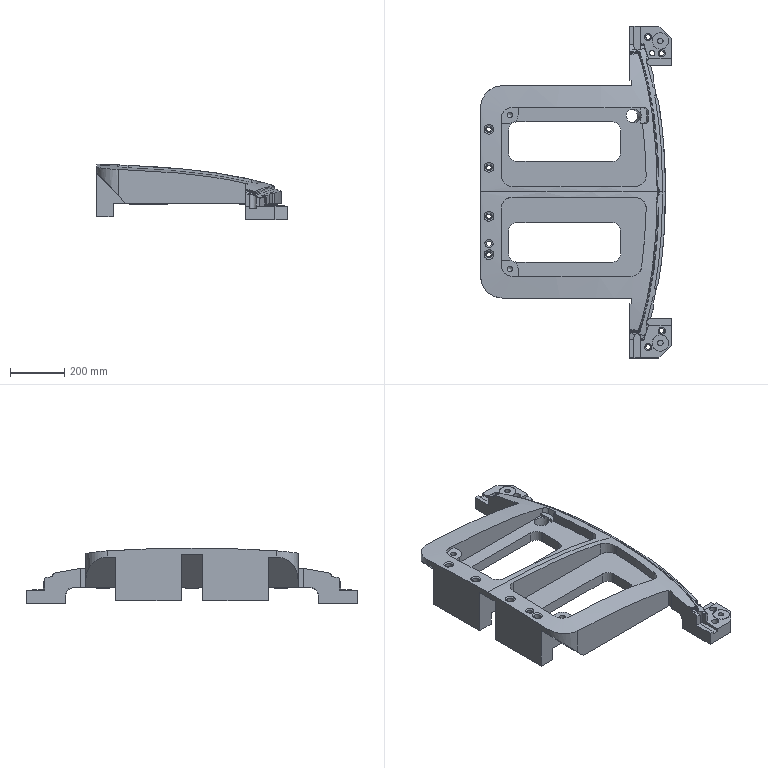Part | NX | features MAIN_BODY 2 | 1 solid | 268 faces | box 700 x 1220 x 203.658 mm | volume 32805003 mm3 | spline 114 | plane 108 | cylinder 44 | cone 2 | commonest cylinder face diameters 60 x12 26 x8 80 x7 17 x4 20 x4 24 x4